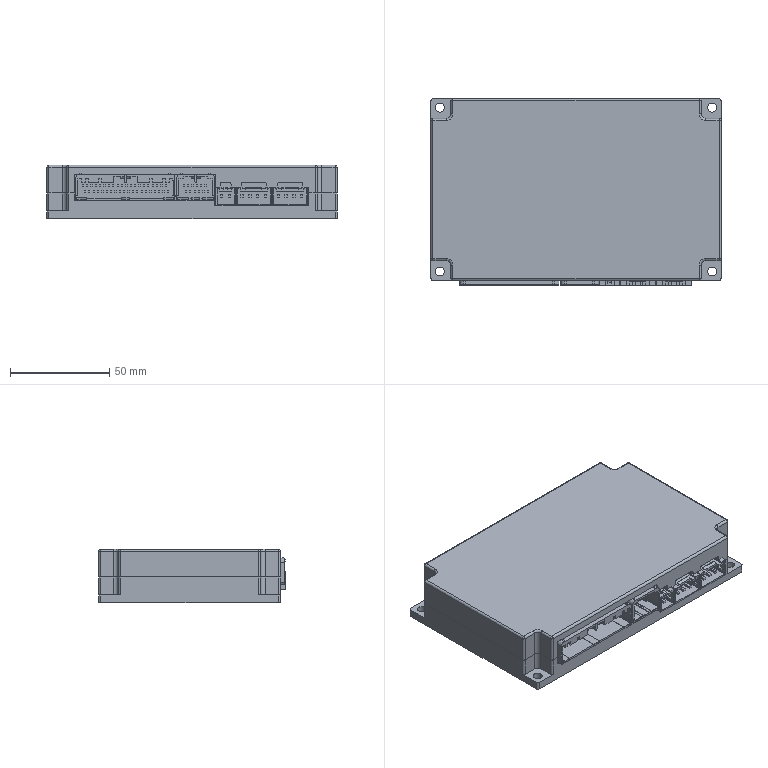Part | NX | features BREP 8 | 8 solids | 1741 faces | box 146 x 94 x 27 mm | volume 100438 mm3 | plane 1461 | cylinder 264 | sphere 8 | torus 4 | cone 4 | commonest cylinder face diameters 2.64 x52 3.92 x52 2 x46 4 x16 5 x14 1 x12